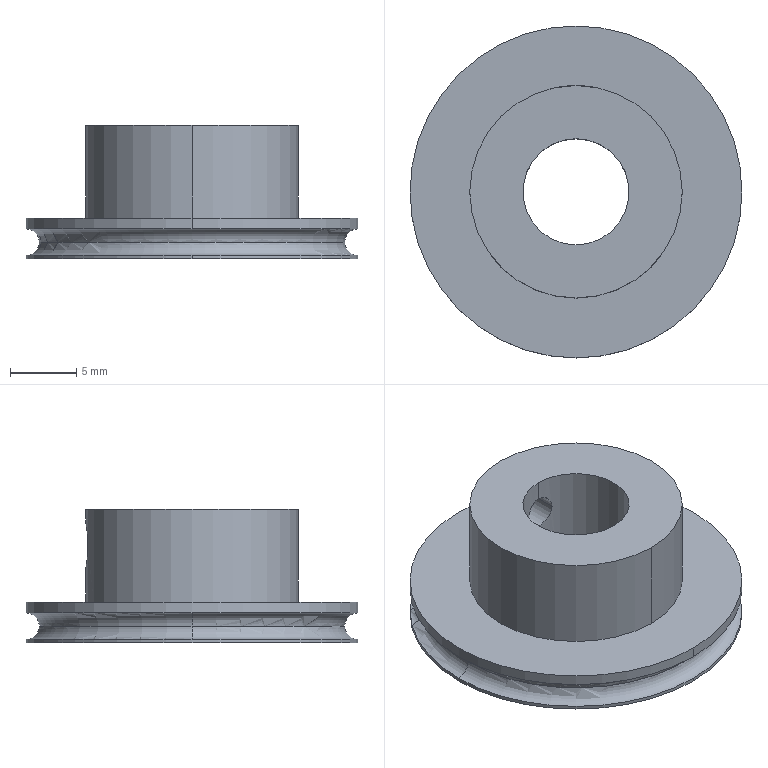Part | NX | 1 solid | 19 faces | box 25 x 25 x 10.05 mm | volume 2260 mm3 | cylinder 10 | torus 4 | plane 3 | spline 2 | commonest cylinder face diameters 25 x4 2.5 x2 8 x2 16 x2